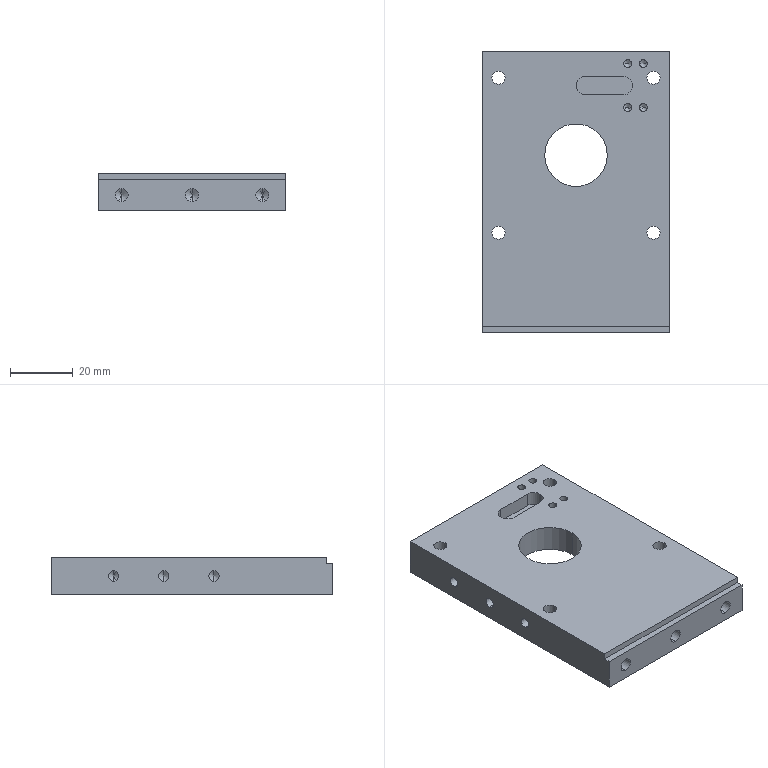Part | SolidWorks | features HoleWzd 7, ICE 5, Chamfer 1, Cut 1, Extrusion 1, MoveFace 1 | 1 solid | 79 faces | box 60 x 90 x 12 mm | volume 52743 mm3 | cylinder 43 | cone 24 | plane 12 | commonest cylinder face diameters 4.2 x14 3.3 x12 2.5 x10 6 x3 20 x2 50.2 x2